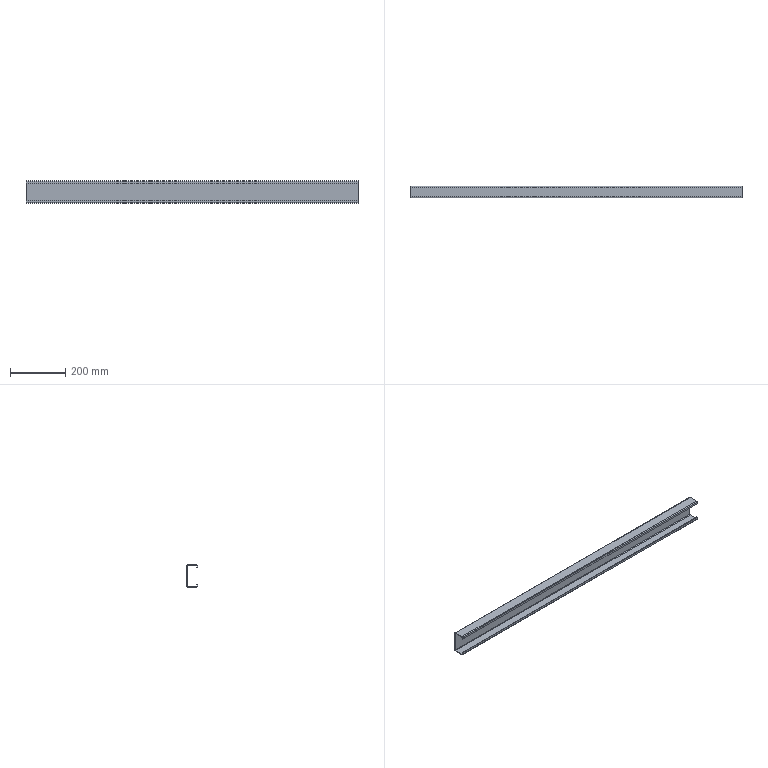Part | SolidWorks | features EdgeFlange 2, FlatPattern 1, SMBaseFlange 1, SheetMetal 1 | 1 solid | 38 faces | box 1200 x 40 x 80 mm | volume 402499 mm3 | plane 30 | cylinder 8 | commonest cylinder face diameters 2 x2 4 x2 6 x2 8 x2
STEP:
#1=CARTESIAN_POINT('',(-1074.379,-37.,-2.));
#2=VERTEX_POINT('',#1);
#3=CARTESIAN_POINT('',(-1074.379,-4.,-2.));
#4=VERTEX_POINT('',#3);
#5=CARTESIAN_POINT('',(-1074.379,0.,-2.));
#6=DIRECTION('',(0.,1.,0.));
#7=VECTOR('',#6,1000.);
#8=LINE('',#5,#7);
#9=EDGE_CURVE('',#2,#4,#8,.T.);
#10=ORIENTED_EDGE('',*,*,#9,.F.);
#11=CARTESIAN_POINT('',(-1074.379,-37.,0.));
#12=VERTEX_POINT('',#11);
#13=CARTESIAN_POINT('',(-1074.379,-37.,-2.));
#14=DIRECTION('',(0.,0.,1.));
#15=VECTOR('',#14,1000.);
#16=LINE('',#13,#15);
#17=EDGE_CURVE('',#2,#12,#16,.T.);
#18=ORIENTED_EDGE('',*,*,#17,.T.);
#19=CARTESIAN_POINT('',(-1074.379,-4.,0.));
#20=VERTEX_POINT('',#19);
#21=CARTESIAN_POINT('',(-1074.379,-2.,0.));
#22=DIRECTION('',(0.,1.,0.));
#23=VECTOR('',#22,1000.);
#24=LINE('',#21,#23);
#25=EDGE_CURVE('',#12,#20,#24,.T.);
#26=ORIENTED_EDGE('',*,*,#25,.T.);
#27=CARTESIAN_POINT('',(-1074.379,-4.,-2.));
#28=DIRECTION('',(0.,0.,1.));
#29=VECTOR('',#28,1000.);
#30=LINE('',#27,#29);
#31=EDGE_CURVE('',#4,#20,#30,.T.);
#32=ORIENTED_EDGE('',*,*,#31,.F.);
#33=EDGE_LOOP('',(#10,#18,#26,#32));
#34=FACE_OUTER_BOUND('',#33,.T.);
#35=CARTESIAN_POINT('',(-1074.379,-2.,0.));
#36=DIRECTION('',(-1.,0.,0.));
#37=DIRECTION('',(0.,0.,1.));
#38=AXIS2_PLACEMENT_3D('',#35,#36,#37);
#39=PLANE('',#38);
#40=ADVANCED_FACE('',(#34),#39,.T.);
#41=ORIENTED_EDGE('',*,*,#25,.F.);
#42=CARTESIAN_POINT('',(125.621,-37.,0.));
#43=VERTEX_POINT('',#42);
#44=CARTESIAN_POINT('',(-1074.379,-37.,0.));
#45=DIRECTION('',(1.,0.,0.));
#46=VECTOR('',#45,1000.);
#47=LINE('',#44,#46);
#48=EDGE_CURVE('',#12,#43,#47,.T.);
#49=ORIENTED_EDGE('',*,*,#48,.T.);
#50=CARTESIAN_POINT('',(125.621,-4.,0.));
#51=VERTEX_POINT('',#50);
#52=CARTESIAN_POINT('',(125.621,-40.,0.));
#53=DIRECTION('',(0.,-1.,0.));
#54=VECTOR('',#53,1000.);
#55=LINE('',#52,#54);
#56=EDGE_CURVE('',#51,#43,#55,.T.);
#57=ORIENTED_EDGE('',*,*,#56,.F.);
#58=CARTESIAN_POINT('',(0.,-4.,0.));
#59=DIRECTION('',(-1.,0.,0.));
#60=VECTOR('',#59,1000.);
#61=LINE('',#58,#60);
#62=EDGE_CURVE('',#51,#20,#61,.T.);
#63=ORIENTED_EDGE('',*,*,#62,.T.);
#64=EDGE_LOOP('',(#41,#49,#57,#63));
#65=FACE_OUTER_BOUND('',#64,.T.);
#66=CARTESIAN_POINT('',(0.,0.,0.));
#67=DIRECTION('',(0.,0.,1.));
#68=DIRECTION('',(0.,-1.,0.));
#69=AXIS2_PLACEMENT_3D('',#66,#67,#68);
#70=PLANE('',#69);
#71=ADVANCED_FACE('',(#65),#70,.T.);
#72=CARTESIAN_POINT('',(125.621,-37.,-2.));
#73=VERTEX_POINT('',#72);
#74=CARTESIAN_POINT('',(-1074.379,-37.,-2.));
#75=DIRECTION('',(1.,0.,0.));
#76=VECTOR('',#75,1000.);
#77=LINE('',#74,#76);
#78=EDGE_CURVE('',#2,#73,#77,.T.);
#79=ORIENTED_EDGE('',*,*,#78,.F.);
#80=ORIENTED_EDGE('',*,*,#9,.T.);
#81=CARTESIAN_POINT('',(125.621,-4.,-2.));
#82=VERTEX_POINT('',#81);
#83=CARTESIAN_POINT('',(125.621,-4.,-2.));
#84=DIRECTION('',(-1.,0.,0.));
#85=VECTOR('',#84,1000.);
#86=LINE('',#83,#85);
#87=EDGE_CURVE('',#82,#4,#86,.T.);
#88=ORIENTED_EDGE('',*,*,#87,.F.);
#89=CARTESIAN_POINT('',(125.621,0.,-2.));
#90=DIRECTION('',(0.,-1.,0.));
#91=VECTOR('',#90,1000.);
#92=LINE('',#89,#91);
#93=EDGE_CURVE('',#82,#73,#92,.T.);
#94=ORIENTED_EDGE('',*,*,#93,.T.);
#95=EDGE_LOOP('',(#79,#80,#88,#94));
#96=FACE_OUTER_BOUND('',#95,.T.);
#97=CARTESIAN_POINT('',(0.,0.,-2.));
#98=DIRECTION('',(0.,0.,1.));
#99=DIRECTION('',(0.,-1.,0.));
#100=AXIS2_PLACEMENT_3D('',#97,#98,#99);
#101=PLANE('',#100);
#102=ADVANCED_FACE('',(#96),#101,.F.);
#103=CARTESIAN_POINT('',(125.621,-37.,-78.));
#104=VERTEX_POINT('',#103);
#105=CARTESIAN_POINT('',(125.621,-4.,-78.));
#106=VERTEX_POINT('',#105);
#107=CARTESIAN_POINT('',(125.621,0.,-78.));
#108=DIRECTION('',(0.,1.,0.));
#109=VECTOR('',#108,1000.);
#110=LINE('',#107,#109);
#111=EDGE_CURVE('',#104,#106,#110,.T.);
#112=ORIENTED_EDGE('',*,*,#111,.F.);
#113=CARTESIAN_POINT('',(125.621,-37.,-80.));
#114=VERTEX_POINT('',#113);
#115=CARTESIAN_POINT('',(125.621,-37.,-78.));
#116=DIRECTION('',(0.,0.,-1.));
#117=VECTOR('',#116,1000.);
#118=LINE('',#115,#117);
#119=EDGE_CURVE('',#104,#114,#118,.T.);
#120=ORIENTED_EDGE('',*,*,#119,.T.);
#121=CARTESIAN_POINT('',(125.621,-4.,-80.));
#122=VERTEX_POINT('',#121);
#123=CARTESIAN_POINT('',(125.621,-2.,-80.));
#124=DIRECTION('',(0.,1.,0.));
#125=VECTOR('',#124,1000.);
#126=LINE('',#123,#125);
#127=EDGE_CURVE('',#114,#122,#126,.T.);
#128=ORIENTED_EDGE('',*,*,#127,.T.);
#129=CARTESIAN_POINT('',(125.621,-4.,-78.));
#130=DIRECTION('',(0.,0.,-1.));
#131=VECTOR('',#130,1000.);
#132=LINE('',#129,#131);
#133=EDGE_CURVE('',#106,#122,#132,.T.);
#134=ORIENTED_EDGE('',*,*,#133,.F.);
#135=EDGE_LOOP('',(#112,#120,#128,#134));
#136=FACE_OUTER_BOUND('',#135,.T.);
#137=CARTESIAN_POINT('',(125.621,-2.,-80.));
#138=DIRECTION('',(1.,0.,0.));
#139=DIRECTION('',(0.,0.,-1.));
#140=AXIS2_PLACEMENT_3D('',#137,#138,#139);
#141=PLANE('',#140);
#142=ADVANCED_FACE('',(#136),#141,.T.);
#143=ORIENTED_EDGE('',*,*,#127,.F.);
#144=CARTESIAN_POINT('',(-1074.379,-37.,-80.));
#145=VERTEX_POINT('',#144);
#146=CARTESIAN_POINT('',(125.621,-37.,-80.));
#147=DIRECTION('',(-1.,0.,0.));
#148=VECTOR('',#147,1000.);
#149=LINE('',#146,#148);
#150=EDGE_CURVE('',#114,#145,#149,.T.);
#151=ORIENTED_EDGE('',*,*,#150,.T.);
#152=CARTESIAN_POINT('',(-1074.379,-4.,-80.));
#153=VERTEX_POINT('',#152);
#154=CARTESIAN_POINT('',(-1074.379,-40.,-80.));
#155=DIRECTION('',(0.,-1.,0.));
#156=VECTOR('',#155,1000.);
#157=LINE('',#154,#156);
#158=EDGE_CURVE('',#153,#145,#157,.T.);
#159=ORIENTED_EDGE('',*,*,#158,.F.);
#160=CARTESIAN_POINT('',(0.,-4.,-80.));
#161=DIRECTION('',(1.,0.,0.));
#162=VECTOR('',#161,1000.);
#163=LINE('',#160,#162);
#164=EDGE_CURVE('',#153,#122,#163,.T.);
#165=ORIENTED_EDGE('',*,*,#164,.T.);
#166=EDGE_LOOP('',(#143,#151,#159,#165));
#167=FACE_OUTER_BOUND('',#166,.T.);
#168=CARTESIAN_POINT('',(0.,0.,-80.));
#169=DIRECTION('',(0.,0.,-1.));
#170=DIRECTION('',(0.,1.,0.));
#171=AXIS2_PLACEMENT_3D('',#168,#169,#170);
#172=PLANE('',#171);
#173=ADVANCED_FACE('',(#167),#172,.T.);
#174=CARTESIAN_POINT('',(-1074.379,-37.,-78.));
#175=VERTEX_POINT('',#174);
#176=CARTESIAN_POINT('',(125.621,-37.,-78.));
#177=DIRECTION('',(-1.,0.,0.));
#178=VECTOR('',#177,1000.);
#179=LINE('',#176,#178);
#180=EDGE_CURVE('',#104,#175,#179,.T.);
#181=ORIENTED_EDGE('',*,*,#180,.F.);
#182=ORIENTED_EDGE('',*,*,#111,.T.);
#183=CARTESIAN_POINT('',(-1074.379,-4.,-78.));
#184=VERTEX_POINT('',#183);
#185=CARTESIAN_POINT('',(-1074.379,-4.,-78.));
#186=DIRECTION('',(1.,0.,0.));
#187=VECTOR('',#186,1000.);
#188=LINE('',#185,#187);
#189=EDGE_CURVE('',#184,#106,#188,.T.);
#190=ORIENTED_EDGE('',*,*,#189,.F.);
#191=CARTESIAN_POINT('',(-1074.379,0.,-78.));
#192=DIRECTION('',(0.,-1.,0.));
#193=VECTOR('',#192,1000.);
#194=LINE('',#191,#193);
#195=EDGE_CURVE('',#184,#175,#194,.T.);
#196=ORIENTED_EDGE('',*,*,#195,.T.);
#197=EDGE_LOOP('',(#181,#182,#190,#196));
#198=FACE_OUTER_BOUND('',#197,.T.);
#199=CARTESIAN_POINT('',(0.,0.,-78.));
#200=DIRECTION('',(0.,0.,-1.));
#201=DIRECTION('',(0.,1.,0.));
#202=AXIS2_PLACEMENT_3D('',#199,#200,#201);
#203=PLANE('',#202);
#204=ADVANCED_FACE('',(#198),#203,.F.);
#205=CARTESIAN_POINT('',(125.621,-2.,-76.));
#206=VERTEX_POINT('',#205);
#207=CARTESIAN_POINT('',(-1074.379,-2.,-76.));
#208=VERTEX_POINT('',#207);
#209=CARTESIAN_POINT('',(125.621,-2.,-76.));
#210=DIRECTION('',(-1.,0.,0.));
#211=VECTOR('',#210,1000.);
#212=LINE('',#209,#211);
#213=EDGE_CURVE('',#206,#208,#212,.T.);
#214=ORIENTED_EDGE('',*,*,#213,.F.);
#215=CARTESIAN_POINT('',(125.621,-2.,-4.));
#216=VERTEX_POINT('',#215);
#217=CARTESIAN_POINT('',(125.621,-2.,-80.));
#218=DIRECTION('',(0.,0.,-1.));
#219=VECTOR('',#218,1000.);
#220=LINE('',#217,#219);
#221=EDGE_CURVE('',#216,#206,#220,.T.);
#222=ORIENTED_EDGE('',*,*,#221,.F.);
#223=CARTESIAN_POINT('',(-1074.379,-2.,-4.));
#224=VERTEX_POINT('',#223);
#225=CARTESIAN_POINT('',(-1074.379,-2.,-4.));
#226=DIRECTION('',(1.,0.,0.));
#227=VECTOR('',#226,1000.);
#228=LINE('',#225,#227);
#229=EDGE_CURVE('',#224,#216,#228,.T.);
#230=ORIENTED_EDGE('',*,*,#229,.F.);
#231=CARTESIAN_POINT('',(-1074.379,-2.,-80.));
#232=DIRECTION('',(0.,0.,1.));
#233=VECTOR('',#232,1000.);
#234=LINE('',#231,#233);
#235=EDGE_CURVE('',#208,#224,#234,.T.);
#236=ORIENTED_EDGE('',*,*,#235,.F.);
#237=EDGE_LOOP('',(#214,#222,#230,#236));
#238=FACE_OUTER_BOUND('',#237,.T.);
#239=CARTESIAN_POINT('',(0.,-2.,0.));
#240=DIRECTION('',(0.,1.,0.));
#241=DIRECTION('',(0.,0.,1.));
#242=AXIS2_PLACEMENT_3D('',#239,#240,#241);
#243=PLANE('',#242);
#244=ADVANCED_FACE('',(#238),#243,.F.);
#245=CARTESIAN_POINT('',(125.621,0.,-4.));
#246=VERTEX_POINT('',#245);
#247=CARTESIAN_POINT('',(125.621,0.,-76.));
#248=VERTEX_POINT('',#247);
#249=CARTESIAN_POINT('',(125.621,0.,-80.));
#250=DIRECTION('',(0.,0.,-1.));
#251=VECTOR('',#250,1000.);
#252=LINE('',#249,#251);
#253=EDGE_CURVE('',#246,#248,#252,.T.);
#254=ORIENTED_EDGE('',*,*,#253,.T.);
#255=CARTESIAN_POINT('',(-1074.379,0.,-76.));
#256=VERTEX_POINT('',#255);
#257=CARTESIAN_POINT('',(125.621,0.,-76.));
#258=DIRECTION('',(-1.,0.,0.));
#259=VECTOR('',#258,1000.);
#260=LINE('',#257,#259);
#261=EDGE_CURVE('',#248,#256,#260,.T.);
#262=ORIENTED_EDGE('',*,*,#261,.T.);
#263=CARTESIAN_POINT('',(-1074.379,0.,-4.));
#264=VERTEX_POINT('',#263);
#265=CARTESIAN_POINT('',(-1074.379,0.,-80.));
#266=DIRECTION('',(0.,0.,1.));
#267=VECTOR('',#266,1000.);
#268=LINE('',#265,#267);
#269=EDGE_CURVE('',#256,#264,#268,.T.);
#270=ORIENTED_EDGE('',*,*,#269,.T.);
#271=CARTESIAN_POINT('',(-1074.379,0.,-4.));
#272=DIRECTION('',(1.,0.,0.));
#273=VECTOR('',#272,1000.);
#274=LINE('',#271,#273);
#275=EDGE_CURVE('',#264,#246,#274,.T.);
#276=ORIENTED_EDGE('',*,*,#275,.T.);
#277=EDGE_LOOP('',(#254,#262,#270,#276));
#278=FACE_OUTER_BOUND('',#277,.T.);
#279=CARTESIAN_POINT('',(0.,0.,0.));
#280=DIRECTION('',(0.,1.,0.));
#281=DIRECTION('',(0.,0.,1.));
#282=AXIS2_PLACEMENT_3D('',#279,#280,#281);
#283=PLANE('',#282);
#284=ADVANCED_FACE('',(#278),#283,.T.);
#285=ORIENTED_EDGE('',*,*,#221,.T.);
#286=CARTESIAN_POINT('',(125.621,-2.,-76.));
#287=DIRECTION('',(0.,1.,0.));
#288=VECTOR('',#287,1000.);
#289=LINE('',#286,#288);
#290=EDGE_CURVE('',#206,#248,#289,.T.);
#291=ORIENTED_EDGE('',*,*,#290,.T.);
#292=ORIENTED_EDGE('',*,*,#253,.F.);
#293=CARTESIAN_POINT('',(125.621,-2.,-4.));
#294=DIRECTION('',(0.,1.,0.));
#295=VECTOR('',#294,1000.);
#296=LINE('',#293,#295);
#297=EDGE_CURVE('',#216,#246,#296,.T.);
#298=ORIENTED_EDGE('',*,*,#297,.F.);
#299=EDGE_LOOP('',(#285,#291,#292,#298));
#300=FACE_OUTER_BOUND('',#299,.T.);
#301=CARTESIAN_POINT('',(125.621,-2.,-80.));
#302=DIRECTION('',(1.,0.,0.));
#303=DIRECTION('',(0.,0.,-1.));
#304=AXIS2_PLACEMENT_3D('',#301,#302,#303);
#305=PLANE('',#304);
#306=ADVANCED_FACE('',(#300),#305,.T.);
#307=CARTESIAN_POINT('',(-1074.379,-2.,-76.));
#308=DIRECTION('',(0.,1.,0.));
#309=VECTOR('',#308,1000.);
#310=LINE('',#307,#309);
#311=EDGE_CURVE('',#208,#256,#310,.T.);
#312=ORIENTED_EDGE('',*,*,#311,.F.);
#313=ORIENTED_EDGE('',*,*,#235,.T.);
#314=CARTESIAN_POINT('',(-1074.379,-2.,-4.));
#315=DIRECTION('',(0.,1.,0.));
#316=VECTOR('',#315,1000.);
#317=LINE('',#314,#316);
#318=EDGE_CURVE('',#224,#264,#317,.T.);
#319=ORIENTED_EDGE('',*,*,#318,.T.);
#320=ORIENTED_EDGE('',*,*,#269,.F.);
#321=EDGE_LOOP('',(#312,#313,#319,#320));
#322=FACE_OUTER_BOUND('',#321,.T.);
#323=CARTESIAN_POINT('',(-1074.379,-2.,-80.));
#324=DIRECTION('',(-1.,0.,0.));
#325=DIRECTION('',(0.,0.,1.));
#326=AXIS2_PLACEMENT_3D('',#323,#324,#325);
#327=PLANE('',#326);
#328=ADVANCED_FACE('',(#322),#327,.T.);
#329=CARTESIAN_POINT('',(125.621,-4.,0.));
#330=DIRECTION('',(0.,0.,1.));
#331=VECTOR('',#330,1000.);
#332=LINE('',#329,#331);
#333=EDGE_CURVE('',#82,#51,#332,.T.);
#334=ORIENTED_EDGE('',*,*,#333,.F.);
#335=CARTESIAN_POINT('',(125.621,-4.,-4.));
#336=DIRECTION('',(1.,0.,0.));
#337=DIRECTION('',(0.,0.,1.));
#338=AXIS2_PLACEMENT_3D('',#335,#336,#337);
#339=CIRCLE('',#338,2.);
#340=EDGE_CURVE('',#216,#82,#339,.T.);
#341=ORIENTED_EDGE('',*,*,#340,.F.);
#342=ORIENTED_EDGE('',*,*,#297,.T.);
#343=CARTESIAN_POINT('',(125.621,-4.,-4.));
#344=DIRECTION('',(1.,0.,0.));
#345=DIRECTION('',(0.,0.,1.));
#346=AXIS2_PLACEMENT_3D('',#343,#344,#345);
#347=CIRCLE('',#346,4.);
#348=EDGE_CURVE('',#246,#51,#347,.T.);
#349=ORIENTED_EDGE('',*,*,#348,.T.);
#350=EDGE_LOOP('',(#334,#341,#342,#349));
#351=FACE_OUTER_BOUND('',#350,.T.);
#352=CARTESIAN_POINT('',(125.621,-4.,-4.));
#353=DIRECTION('',(1.,0.,0.));
#354=DIRECTION('',(0.,0.,-1.));
#355=AXIS2_PLACEMENT_3D('',#352,#353,#354);
#356=PLANE('',#355);
#357=ADVANCED_FACE('',(#351),#356,.T.);
#358=CARTESIAN_POINT('',(-1074.379,-4.,-4.));
#359=DIRECTION('',(-1.,0.,0.));
#360=DIRECTION('',(0.,0.,1.));
#361=AXIS2_PLACEMENT_3D('',#358,#359,#360);
#362=CIRCLE('',#361,2.);
#363=EDGE_CURVE('',#4,#224,#362,.T.);
#364=ORIENTED_EDGE('',*,*,#363,.F.);
#365=ORIENTED_EDGE('',*,*,#31,.T.);
#366=CARTESIAN_POINT('',(-1074.379,-4.,-4.));
#367=DIRECTION('',(-1.,0.,0.));
#368=DIRECTION('',(0.,0.,1.));
#369=AXIS2_PLACEMENT_3D('',#366,#367,#368);
#370=CIRCLE('',#369,4.);
#371=EDGE_CURVE('',#20,#264,#370,.T.);
#372=ORIENTED_EDGE('',*,*,#371,.T.);
#373=ORIENTED_EDGE('',*,*,#318,.F.);
#374=EDGE_LOOP('',(#364,#365,#372,#373));
#375=FACE_OUTER_BOUND('',#374,.T.);
#376=CARTESIAN_POINT('',(-1074.379,-4.,-4.));
#377=DIRECTION('',(1.,0.,0.));
#378=DIRECTION('',(0.,0.,-1.));
#379=AXIS2_PLACEMENT_3D('',#376,#377,#378);
#380=PLANE('',#379);
#381=ADVANCED_FACE('',(#375),#380,.F.);
#382=ORIENTED_EDGE('',*,*,#275,.F.);
#383=ORIENTED_EDGE('',*,*,#371,.F.);
#384=ORIENTED_EDGE('',*,*,#62,.F.);
#385=ORIENTED_EDGE('',*,*,#348,.F.);
#386=EDGE_LOOP('',(#382,#383,#384,#385));
#387=FACE_OUTER_BOUND('',#386,.T.);
#388=CARTESIAN_POINT('',(-1074.379,-4.,-4.));
#389=DIRECTION('',(-1.,0.,0.));
#390=DIRECTION('',(0.,0.,1.));
#391=AXIS2_PLACEMENT_3D('',#388,#389,#390);
#392=CYLINDRICAL_SURFACE('',#391,4.);
#393=ADVANCED_FACE('',(#387),#392,.T.);
#394=ORIENTED_EDGE('',*,*,#229,.T.);
#395=ORIENTED_EDGE('',*,*,#340,.T.);
#396=ORIENTED_EDGE('',*,*,#87,.T.);
#397=ORIENTED_EDGE('',*,*,#363,.T.);
#398=EDGE_LOOP('',(#394,#395,#396,#397));
#399=FACE_OUTER_BOUND('',#398,.T.);
#400=CARTESIAN_POINT('',(-1074.379,-4.,-4.));
#401=DIRECTION('',(-1.,0.,0.));
#402=DIRECTION('',(0.,0.,1.));
#403=AXIS2_PLACEMENT_3D('',#400,#401,#402);
#404=CYLINDRICAL_SURFACE('',#403,2.);
#405=ADVANCED_FACE('',(#399),#404,.F.);
#406=CARTESIAN_POINT('',(125.621,-37.,-2.));
#407=DIRECTION('',(0.,0.,1.));
#408=VECTOR('',#407,1000.);
#409=LINE('',#406,#408);
#410=EDGE_CURVE('',#73,#43,#409,.T.);
#411=ORIENTED_EDGE('',*,*,#410,.F.);
#412=ORIENTED_EDGE('',*,*,#93,.F.);
#413=ORIENTED_EDGE('',*,*,#333,.T.);
#414=ORIENTED_EDGE('',*,*,#56,.T.);
#415=EDGE_LOOP('',(#411,#412,#413,#414));
#416=FACE_OUTER_BOUND('',#415,.T.);
#417=CARTESIAN_POINT('',(125.621,-40.,0.));
#418=DIRECTION('',(1.,0.,0.));
#419=DIRECTION('',(0.,0.,-1.));
#420=AXIS2_PLACEMENT_3D('',#417,#418,#419);
#421=PLANE('',#420);
#422=ADVANCED_FACE('',(#416),#421,.T.);
#423=CARTESIAN_POINT('',(-1074.379,-4.,-80.));
#424=DIRECTION('',(0.,0.,-1.));
#425=VECTOR('',#424,1000.);
#426=LINE('',#423,#425);
#427=EDGE_CURVE('',#184,#153,#426,.T.);
#428=ORIENTED_EDGE('',*,*,#427,.F.);
#429=CARTESIAN_POINT('',(-1074.379,-4.,-76.));
#430=DIRECTION('',(-1.,0.,0.));
#431=DIRECTION('',(0.,0.,-1.));
#432=AXIS2_PLACEMENT_3D('',#429,#430,#431);
#433=CIRCLE('',#432,2.);
#434=EDGE_CURVE('',#208,#184,#433,.T.);
#435=ORIENTED_EDGE('',*,*,#434,.F.);
#436=ORIENTED_EDGE('',*,*,#311,.T.);
#437=CARTESIAN_POINT('',(-1074.379,-4.,-76.));
#438=DIRECTION('',(-1.,0.,0.));
#439=DIRECTION('',(0.,0.,-1.));
#440=AXIS2_PLACEMENT_3D('',#437,#438,#439);
#441=CIRCLE('',#440,4.);
#442=EDGE_CURVE('',#256,#153,#441,.T.);
#443=ORIENTED_EDGE('',*,*,#442,.T.);
#444=EDGE_LOOP('',(#428,#435,#436,#443));
#445=FACE_OUTER_BOUND('',#444,.T.);
#446=CARTESIAN_POINT('',(-1074.379,-4.,-76.));
#447=DIRECTION('',(-1.,0.,0.));
#448=DIRECTION('',(0.,0.,1.));
#449=AXIS2_PLACEMENT_3D('',#446,#447,#448);
#450=PLANE('',#449);
#451=ADVANCED_FACE('',(#445),#450,.T.);
#452=CARTESIAN_POINT('',(125.621,-4.,-76.));
#453=DIRECTION('',(1.,0.,0.));
#454=DIRECTION('',(0.,0.,-1.));
#455=AXIS2_PLACEMENT_3D('',#452,#453,#454);
#456=CIRCLE('',#455,2.);
#457=EDGE_CURVE('',#106,#206,#456,.T.);
#458=ORIENTED_EDGE('',*,*,#457,.F.);
#459=ORIENTED_EDGE('',*,*,#133,.T.);
#460=CARTESIAN_POINT('',(125.621,-4.,-76.));
#461=DIRECTION('',(1.,0.,0.));
#462=DIRECTION('',(0.,0.,-1.));
#463=AXIS2_PLACEMENT_3D('',#460,#461,#462);
#464=CIRCLE('',#463,4.);
#465=EDGE_CURVE('',#122,#248,#464,.T.);
#466=ORIENTED_EDGE('',*,*,#465,.T.);
#467=ORIENTED_EDGE('',*,*,#290,.F.);
#468=EDGE_LOOP('',(#458,#459,#466,#467));
#469=FACE_OUTER_BOUND('',#468,.T.);
#470=CARTESIAN_POINT('',(125.621,-4.,-76.));
#471=DIRECTION('',(-1.,0.,0.));
#472=DIRECTION('',(0.,0.,1.));
#473=AXIS2_PLACEMENT_3D('',#470,#471,#472);
#474=PLANE('',#473);
#475=ADVANCED_FACE('',(#469),#474,.F.);
#476=ORIENTED_EDGE('',*,*,#261,.F.);
#477=ORIENTED_EDGE('',*,*,#465,.F.);
#478=ORIENTED_EDGE('',*,*,#164,.F.);
#479=ORIENTED_EDGE('',*,*,#442,.F.);
#480=EDGE_LOOP('',(#476,#477,#478,#479));
#481=FACE_OUTER_BOUND('',#480,.T.);
#482=CARTESIAN_POINT('',(125.621,-4.,-76.));
#483=DIRECTION('',(1.,0.,0.));
#484=DIRECTION('',(0.,0.,-1.));
#485=AXIS2_PLACEMENT_3D('',#482,#483,#484);
#486=CYLINDRICAL_SURFACE('',#485,4.);
#487=ADVANCED_FACE('',(#481),#486,.T.);
#488=ORIENTED_EDGE('',*,*,#213,.T.);
#489=ORIENTED_EDGE('',*,*,#434,.T.);
#490=ORIENTED_EDGE('',*,*,#189,.T.);
#491=ORIENTED_EDGE('',*,*,#457,.T.);
#492=EDGE_LOOP('',(#488,#489,#490,#491));
#493=FACE_OUTER_BOUND('',#492,.T.);
#494=CARTESIAN_POINT('',(125.621,-4.,-76.));
#495=DIRECTION('',(1.,0.,0.));
#496=DIRECTION('',(0.,0.,-1.));
#497=AXIS2_PLACEMENT_3D('',#494,#495,#496);
#498=CYLINDRICAL_SURFACE('',#497,2.);
#499=ADVANCED_FACE('',(#493),#498,.F.);
#500=CARTESIAN_POINT('',(-1074.379,-37.,-78.));
#501=DIRECTION('',(0.,0.,-1.));
#502=VECTOR('',#501,1000.);
#503=LINE('',#500,#502);
#504=EDGE_CURVE('',#175,#145,#503,.T.);
#505=ORIENTED_EDGE('',*,*,#504,.F.);
#506=ORIENTED_EDGE('',*,*,#195,.F.);
#507=ORIENTED_EDGE('',*,*,#427,.T.);
#508=ORIENTED_EDGE('',*,*,#158,.T.);
#509=EDGE_LOOP('',(#505,#506,#507,#508));
#510=FACE_OUTER_BOUND('',#509,.T.);
#511=CARTESIAN_POINT('',(-1074.379,-40.,-80.));
#512=DIRECTION('',(-1.,0.,0.));
#513=DIRECTION('',(0.,0.,1.));
#514=AXIS2_PLACEMENT_3D('',#511,#512,#513);
#515=PLANE('',#514);
#516=ADVANCED_FACE('',(#510),#515,.T.);
#517=CARTESIAN_POINT('',(-1074.379,-38.,-77.));
#518=VERTEX_POINT('',#517);
#519=CARTESIAN_POINT('',(-1074.379,-40.,-77.));
#520=VERTEX_POINT('',#519);
#521=CARTESIAN_POINT('',(-1074.379,-40.,-77.));
#522=DIRECTION('',(0.,-1.,0.));
#523=VECTOR('',#522,1000.);
#524=LINE('',#521,#523);
#525=EDGE_CURVE('',#518,#520,#524,.T.);
#526=ORIENTED_EDGE('',*,*,#525,.F.);
#527=CARTESIAN_POINT('',(-1074.379,-37.,-77.));
#528=DIRECTION('',(-1.,0.,0.));
#529=DIRECTION('',(0.,0.,-1.));
#530=AXIS2_PLACEMENT_3D('',#527,#528,#529);
#531=CIRCLE('',#530,1.);
#532=EDGE_CURVE('',#175,#518,#531,.T.);
#533=ORIENTED_EDGE('',*,*,#532,.F.);
#534=ORIENTED_EDGE('',*,*,#504,.T.);
#535=CARTESIAN_POINT('',(-1074.379,-37.,-77.));
#536=DIRECTION('',(-1.,0.,0.));
#537=DIRECTION('',(0.,0.,-1.));
#538=AXIS2_PLACEMENT_3D('',#535,#536,#537);
#539=CIRCLE('',#538,3.);
#540=EDGE_CURVE('',#145,#520,#539,.T.);
#541=ORIENTED_EDGE('',*,*,#540,.T.);
#542=EDGE_LOOP('',(#526,#533,#534,#541));
#543=FACE_OUTER_BOUND('',#542,.T.);
#544=CARTESIAN_POINT('',(-1074.379,-37.,-77.));
#545=DIRECTION('',(-1.,0.,0.));
#546=DIRECTION('',(0.,0.,1.));
#547=AXIS2_PLACEMENT_3D('',#544,#545,#546);
#548=PLANE('',#547);
#549=ADVANCED_FACE('',(#543),#548,.T.);
#550=CARTESIAN_POINT('',(125.621,-38.,-77.));
#551=VERTEX_POINT('',#550);
#552=CARTESIAN_POINT('',(125.621,-37.,-77.));
#553=DIRECTION('',(1.,0.,0.));
#554=DIRECTION('',(0.,0.,-1.));
#555=AXIS2_PLACEMENT_3D('',#552,#553,#554);
#556=CIRCLE('',#555,1.);
#557=EDGE_CURVE('',#551,#104,#556,.T.);
#558=ORIENTED_EDGE('',*,*,#557,.F.);
#559=CARTESIAN_POINT('',(125.621,-40.,-77.));
#560=VERTEX_POINT('',#559);
#561=CARTESIAN_POINT('',(125.621,-38.,-77.));
#562=DIRECTION('',(0.,-1.,0.));
#563=VECTOR('',#562,1000.);
#564=LINE('',#561,#563);
#565=EDGE_CURVE('',#551,#560,#564,.T.);
#566=ORIENTED_EDGE('',*,*,#565,.T.);
#567=CARTESIAN_POINT('',(125.621,-37.,-77.));
#568=DIRECTION('',(1.,0.,0.));
#569=DIRECTION('',(0.,0.,-1.));
#570=AXIS2_PLACEMENT_3D('',#567,#568,#569);
#571=CIRCLE('',#570,3.);
#572=EDGE_CURVE('',#560,#114,#571,.T.);
#573=ORIENTED_EDGE('',*,*,#572,.T.);
#574=ORIENTED_EDGE('',*,*,#119,.F.);
#575=EDGE_LOOP('',(#558,#566,#573,#574));
#576=FACE_OUTER_BOUND('',#575,.T.);
#577=CARTESIAN_POINT('',(125.621,-37.,-77.));
#578=DIRECTION('',(-1.,0.,0.));
#579=DIRECTION('',(0.,0.,1.));
#580=AXIS2_PLACEMENT_3D('',#577,#578,#579);
#581=PLANE('',#580);
#582=ADVANCED_FACE('',(#576),#581,.F.);
#583=ORIENTED_EDGE('',*,*,#150,.F.);
#584=ORIENTED_EDGE('',*,*,#572,.F.);
#585=CARTESIAN_POINT('',(-1074.379,-40.,-77.));
#586=DIRECTION('',(-1.,0.,0.));
#587=VECTOR('',#586,1000.);
#588=LINE('',#585,#587);
#589=EDGE_CURVE('',#560,#520,#588,.T.);
#590=ORIENTED_EDGE('',*,*,#589,.T.);
#591=ORIENTED_EDGE('',*,*,#540,.F.);
#592=EDGE_LOOP('',(#583,#584,#590,#591));
#593=FACE_OUTER_BOUND('',#592,.T.);
#594=CARTESIAN_POINT('',(125.621,-37.,-77.));
#595=DIRECTION('',(1.,0.,0.));
#596=DIRECTION('',(0.,-1.,0.));
#597=AXIS2_PLACEMENT_3D('',#594,#595,#596);
#598=CYLINDRICAL_SURFACE('',#597,3.);
#599=ADVANCED_FACE('',(#593),#598,.T.);
#600=ORIENTED_EDGE('',*,*,#180,.T.);
#601=ORIENTED_EDGE('',*,*,#532,.T.);
#602=CARTESIAN_POINT('',(-1074.379,-38.,-77.));
#603=DIRECTION('',(1.,0.,0.));
#604=VECTOR('',#603,1000.);
#605=LINE('',#602,#604);
#606=EDGE_CURVE('',#518,#551,#605,.T.);
#607=ORIENTED_EDGE('',*,*,#606,.T.);
#608=ORIENTED_EDGE('',*,*,#557,.T.);
#609=EDGE_LOOP('',(#600,#601,#607,#608));
#610=FACE_OUTER_BOUND('',#609,.T.);
#611=CARTESIAN_POINT('',(125.621,-37.,-77.));
#612=DIRECTION('',(1.,0.,0.));
#613=DIRECTION('',(0.,-1.,0.));
#614=AXIS2_PLACEMENT_3D('',#611,#612,#613);
#615=CYLINDRICAL_SURFACE('',#614,1.);
#616=ADVANCED_FACE('',(#610),#615,.F.);
#617=ORIENTED_EDGE('',*,*,#565,.F.);
#618=CARTESIAN_POINT('',(125.621,-38.,-70.));
#619=VERTEX_POINT('',#618);
#620=CARTESIAN_POINT('',(125.621,-38.,-70.));
#621=DIRECTION('',(0.,0.,1.));
#622=VECTOR('',#621,1000.);
#623=LINE('',#620,#622);
#624=EDGE_CURVE('',#551,#619,#623,.T.);
#625=ORIENTED_EDGE('',*,*,#624,.T.);
#626=CARTESIAN_POINT('',(125.621,-40.,-70.));
#627=VERTEX_POINT('',#626);
#628=CARTESIAN_POINT('',(125.621,-40.,-70.));
#629=DIRECTION('',(0.,1.,0.));
#630=VECTOR('',#629,1000.);
#631=LINE('',#628,#630);
#632=EDGE_CURVE('',#627,#619,#631,.T.);
#633=ORIENTED_EDGE('',*,*,#632,.F.);
#634=CARTESIAN_POINT('',(125.621,-40.,0.));
#635=DIRECTION('',(0.,0.,1.));
#636=VECTOR('',#635,1000.);
#637=LINE('',#634,#636);
#638=EDGE_CURVE('',#560,#627,#637,.T.);
#639=ORIENTED_EDGE('',*,*,#638,.F.);
#640=EDGE_LOOP('',(#617,#625,#633,#639));
#641=FACE_OUTER_BOUND('',#640,.T.);
#642=CARTESIAN_POINT('',(125.621,-40.,-70.));
#643=DIRECTION('',(-1.,0.,0.));
#644=DIRECTION('',(0.,-1.,0.));
#645=AXIS2_PLACEMENT_3D('',#642,#643,#644);
#646=PLANE('',#645);
#647=ADVANCED_FACE('',(#641),#646,.F.);
#648=ORIENTED_EDGE('',*,*,#525,.T.);
#649=CARTESIAN_POINT('',(-1074.379,-40.,-70.));
#650=VERTEX_POINT('',#649);
#651=CARTESIAN_POINT('',(-1074.379,-40.,0.));
#652=DIRECTION('',(0.,0.,-1.));
#653=VECTOR('',#652,1000.);
#654=LINE('',#651,#653);
#655=EDGE_CURVE('',#650,#520,#654,.T.);
#656=ORIENTED_EDGE('',*,*,#655,.F.);
#657=CARTESIAN_POINT('',(-1074.379,-38.,-70.));
#658=VERTEX_POINT('',#657);
#659=CARTESIAN_POINT('',(-1074.379,-40.,-70.));
#660=DIRECTION('',(0.,1.,0.));
#661=VECTOR('',#660,1000.);
#662=LINE('',#659,#661);
#663=EDGE_CURVE('',#650,#658,#662,.T.);
#664=ORIENTED_EDGE('',*,*,#663,.T.);
#665=CARTESIAN_POINT('',(-1074.379,-38.,-78.));
#666=DIRECTION('',(0.,0.,-1.));
#667=VECTOR('',#666,1000.);
#668=LINE('',#665,#667);
#669=EDGE_CURVE('',#658,#518,#668,.T.);
#670=ORIENTED_EDGE('',*,*,#669,.T.);
#671=EDGE_LOOP('',(#648,#656,#664,#670));
#672=FACE_OUTER_BOUND('',#671,.T.);
#673=CARTESIAN_POINT('',(-1074.379,-40.,-78.));
#674=DIRECTION('',(1.,0.,0.));
#675=DIRECTION('',(0.,1.,0.));
#676=AXIS2_PLACEMENT_3D('',#673,#674,#675);
#677=PLANE('',#676);
#678=ADVANCED_FACE('',(#672),#677,.F.);
#679=ORIENTED_EDGE('',*,*,#589,.F.);
#680=ORIENTED_EDGE('',*,*,#638,.T.);
#681=CARTESIAN_POINT('',(0.,-40.,-70.));
#682=DIRECTION('',(-1.,0.,0.));
#683=VECTOR('',#682,1000.);
#684=LINE('',#681,#683);
#685=EDGE_CURVE('',#627,#650,#684,.T.);
#686=ORIENTED_EDGE('',*,*,#685,.T.);
#687=ORIENTED_EDGE('',*,*,#655,.T.);
#688=EDGE_LOOP('',(#679,#680,#686,#687));
#689=FACE_OUTER_BOUND('',#688,.T.);
#690=CARTESIAN_POINT('',(0.,-40.,0.));
#691=DIRECTION('',(0.,1.,0.));
#692=DIRECTION('',(0.,0.,1.));
#693=AXIS2_PLACEMENT_3D('',#690,#691,#692);
#694=PLANE('',#693);
#695=ADVANCED_FACE('',(#689),#694,.F.);
#696=ORIENTED_EDGE('',*,*,#624,.F.);
#697=ORIENTED_EDGE('',*,*,#606,.F.);
#698=ORIENTED_EDGE('',*,*,#669,.F.);
#699=CARTESIAN_POINT('',(-1074.379,-38.,-70.));
#700=DIRECTION('',(-1.,0.,0.));
#701=VECTOR('',#700,1000.);
#702=LINE('',#699,#701);
#703=EDGE_CURVE('',#619,#658,#702,.T.);
#704=ORIENTED_EDGE('',*,*,#703,.F.);
#705=EDGE_LOOP('',(#696,#697,#698,#704));
#706=FACE_OUTER_BOUND('',#705,.T.);
#707=CARTESIAN_POINT('',(0.,-38.,0.));
#708=DIRECTION('',(0.,1.,0.));
#709=DIRECTION('',(0.,0.,1.));
#710=AXIS2_PLACEMENT_3D('',#707,#708,#709);
#711=PLANE('',#710);
#712=ADVANCED_FACE('',(#706),#711,.T.);
#713=ORIENTED_EDGE('',*,*,#703,.T.);
#714=ORIENTED_EDGE('',*,*,#663,.F.);
#715=ORIENTED_EDGE('',*,*,#685,.F.);
#716=ORIENTED_EDGE('',*,*,#632,.T.);
#717=EDGE_LOOP('',(#713,#714,#715,#716));
#718=FACE_OUTER_BOUND('',#717,.T.);
#719=CARTESIAN_POINT('',(-1074.379,-40.,-70.));
#720=DIRECTION('',(0.,0.,-1.));
#721=DIRECTION('',(0.,1.,0.));
#722=AXIS2_PLACEMENT_3D('',#719,#720,#721);
#723=PLANE('',#722);
#724=ADVANCED_FACE('',(#718),#723,.F.);
#725=CARTESIAN_POINT('',(125.621,-38.,-3.));
#726=VERTEX_POINT('',#725);
#727=CARTESIAN_POINT('',(125.621,-40.,-3.));
#728=VERTEX_POINT('',#727);
#729=CARTESIAN_POINT('',(125.621,-40.,-3.));
#730=DIRECTION('',(0.,-1.,0.));
#731=VECTOR('',#730,1000.);
#732=LINE('',#729,#731);
#733=EDGE_CURVE('',#726,#728,#732,.T.);
#734=ORIENTED_EDGE('',*,*,#733,.F.);
#735=CARTESIAN_POINT('',(125.621,-37.,-3.));
#736=DIRECTION('',(1.,0.,0.));
#737=DIRECTION('',(0.,0.,1.));
#738=AXIS2_PLACEMENT_3D('',#735,#736,#737);
#739=CIRCLE('',#738,1.);
#740=EDGE_CURVE('',#73,#726,#739,.T.);
#741=ORIENTED_EDGE('',*,*,#740,.F.);
#742=ORIENTED_EDGE('',*,*,#410,.T.);
#743=CARTESIAN_POINT('',(125.621,-37.,-3.));
#744=DIRECTION('',(1.,0.,0.));
#745=DIRECTION('',(0.,0.,1.));
#746=AXIS2_PLACEMENT_3D('',#743,#744,#745);
#747=CIRCLE('',#746,3.);
#748=EDGE_CURVE('',#43,#728,#747,.T.);
#749=ORIENTED_EDGE('',*,*,#748,.T.);
#750=EDGE_LOOP('',(#734,#741,#742,#749));
#751=FACE_OUTER_BOUND('',#750,.T.);
#752=CARTESIAN_POINT('',(125.621,-37.,-3.));
#753=DIRECTION('',(1.,0.,0.));
#754=DIRECTION('',(0.,0.,-1.));
#755=AXIS2_PLACEMENT_3D('',#752,#753,#754);
#756=PLANE('',#755);
#757=ADVANCED_FACE('',(#751),#756,.T.);
#758=CARTESIAN_POINT('',(-1074.379,-38.,-3.));
#759=VERTEX_POINT('',#758);
#760=CARTESIAN_POINT('',(-1074.379,-37.,-3.));
#761=DIRECTION('',(-1.,0.,0.));
#762=DIRECTION('',(0.,0.,1.));
#763=AXIS2_PLACEMENT_3D('',#760,#761,#762);
#764=CIRCLE('',#763,1.);
#765=EDGE_CURVE('',#759,#2,#764,.T.);
#766=ORIENTED_EDGE('',*,*,#765,.F.);
#767=CARTESIAN_POINT('',(-1074.379,-40.,-3.));
#768=VERTEX_POINT('',#767);
#769=CARTESIAN_POINT('',(-1074.379,-38.,-3.));
#770=DIRECTION('',(0.,-1.,0.));
#771=VECTOR('',#770,1000.);
#772=LINE('',#769,#771);
#773=EDGE_CURVE('',#759,#768,#772,.T.);
#774=ORIENTED_EDGE('',*,*,#773,.T.);
#775=CARTESIAN_POINT('',(-1074.379,-37.,-3.));
#776=DIRECTION('',(-1.,0.,0.));
#777=DIRECTION('',(0.,0.,1.));
#778=AXIS2_PLACEMENT_3D('',#775,#776,#777);
#779=CIRCLE('',#778,3.);
#780=EDGE_CURVE('',#768,#12,#779,.T.);
#781=ORIENTED_EDGE('',*,*,#780,.T.);
#782=ORIENTED_EDGE('',*,*,#17,.F.);
#783=EDGE_LOOP('',(#766,#774,#781,#782));
#784=FACE_OUTER_BOUND('',#783,.T.);
#785=CARTESIAN_POINT('',(-1074.379,-37.,-3.));
#786=DIRECTION('',(1.,0.,0.));
#787=DIRECTION('',(0.,0.,-1.));
#788=AXIS2_PLACEMENT_3D('',#785,#786,#787);
#789=PLANE('',#788);
#790=ADVANCED_FACE('',(#784),#789,.F.);
#791=ORIENTED_EDGE('',*,*,#48,.F.);
#792=ORIENTED_EDGE('',*,*,#780,.F.);
#793=CARTESIAN_POINT('',(125.621,-40.,-3.));
#794=DIRECTION('',(1.,0.,0.));
#795=VECTOR('',#794,1000.);
#796=LINE('',#793,#795);
#797=EDGE_CURVE('',#768,#728,#796,.T.);
#798=ORIENTED_EDGE('',*,*,#797,.T.);
#799=ORIENTED_EDGE('',*,*,#748,.F.);
#800=EDGE_LOOP('',(#791,#792,#798,#799));
#801=FACE_OUTER_BOUND('',#800,.T.);
#802=CARTESIAN_POINT('',(-1074.379,-37.,-3.));
#803=DIRECTION('',(-1.,0.,0.));
#804=DIRECTION('',(0.,-1.,0.));
#805=AXIS2_PLACEMENT_3D('',#802,#803,#804);
#806=CYLINDRICAL_SURFACE('',#805,3.);
#807=ADVANCED_FACE('',(#801),#806,.T.);
#808=ORIENTED_EDGE('',*,*,#78,.T.);
#809=ORIENTED_EDGE('',*,*,#740,.T.);
#810=CARTESIAN_POINT('',(125.621,-38.,-3.));
#811=DIRECTION('',(-1.,0.,0.));
#812=VECTOR('',#811,1000.);
#813=LINE('',#810,#812);
#814=EDGE_CURVE('',#726,#759,#813,.T.);
#815=ORIENTED_EDGE('',*,*,#814,.T.);
#816=ORIENTED_EDGE('',*,*,#765,.T.);
#817=EDGE_LOOP('',(#808,#809,#815,#816));
#818=FACE_OUTER_BOUND('',#817,.T.);
#819=CARTESIAN_POINT('',(-1074.379,-37.,-3.));
#820=DIRECTION('',(-1.,0.,0.));
#821=DIRECTION('',(0.,-1.,0.));
#822=AXIS2_PLACEMENT_3D('',#819,#820,#821);
#823=CYLINDRICAL_SURFACE('',#822,1.);
#824=ADVANCED_FACE('',(#818),#823,.F.);
#825=ORIENTED_EDGE('',*,*,#733,.T.);
#826=CARTESIAN_POINT('',(125.621,-40.,-10.));
#827=VERTEX_POINT('',#826);
#828=CARTESIAN_POINT('',(125.621,-40.,0.));
#829=DIRECTION('',(0.,0.,1.));
#830=VECTOR('',#829,1000.);
#831=LINE('',#828,#830);
#832=EDGE_CURVE('',#827,#728,#831,.T.);
#833=ORIENTED_EDGE('',*,*,#832,.F.);
#834=CARTESIAN_POINT('',(125.621,-38.,-10.));
#835=VERTEX_POINT('',#834);
#836=CARTESIAN_POINT('',(125.621,-40.,-10.));
#837=DIRECTION('',(0.,1.,0.));
#838=VECTOR('',#837,1000.);
#839=LINE('',#836,#838);
#840=EDGE_CURVE('',#827,#835,#839,.T.);
#841=ORIENTED_EDGE('',*,*,#840,.T.);
#842=CARTESIAN_POINT('',(125.621,-38.,-2.));
#843=DIRECTION('',(0.,0.,1.));
#844=VECTOR('',#843,1000.);
#845=LINE('',#842,#844);
#846=EDGE_CURVE('',#835,#726,#845,.T.);
#847=ORIENTED_EDGE('',*,*,#846,.T.);
#848=EDGE_LOOP('',(#825,#833,#841,#847));
#849=FACE_OUTER_BOUND('',#848,.T.);
#850=CARTESIAN_POINT('',(125.621,-40.,-2.));
#851=DIRECTION('',(-1.,0.,0.));
#852=DIRECTION('',(0.,0.,1.));
#853=AXIS2_PLACEMENT_3D('',#850,#851,#852);
#854=PLANE('',#853);
#855=ADVANCED_FACE('',(#849),#854,.F.);
#856=ORIENTED_EDGE('',*,*,#773,.F.);
#857=CARTESIAN_POINT('',(-1074.379,-38.,-10.));
#858=VERTEX_POINT('',#857);
#859=CARTESIAN_POINT('',(-1074.379,-38.,-10.));
#860=DIRECTION('',(0.,0.,-1.));
#861=VECTOR('',#860,1000.);
#862=LINE('',#859,#861);
#863=EDGE_CURVE('',#759,#858,#862,.T.);
#864=ORIENTED_EDGE('',*,*,#863,.T.);
#865=CARTESIAN_POINT('',(-1074.379,-40.,-10.));
#866=VERTEX_POINT('',#865);
#867=CARTESIAN_POINT('',(-1074.379,-40.,-10.));
#868=DIRECTION('',(0.,1.,0.));
#869=VECTOR('',#868,1000.);
#870=LINE('',#867,#869);
#871=EDGE_CURVE('',#866,#858,#870,.T.);
#872=ORIENTED_EDGE('',*,*,#871,.F.);
#873=CARTESIAN_POINT('',(-1074.379,-40.,0.));
#874=DIRECTION('',(0.,0.,-1.));
#875=VECTOR('',#874,1000.);
#876=LINE('',#873,#875);
#877=EDGE_CURVE('',#768,#866,#876,.T.);
#878=ORIENTED_EDGE('',*,*,#877,.F.);
#879=EDGE_LOOP('',(#856,#864,#872,#878));
#880=FACE_OUTER_BOUND('',#879,.T.);
#881=CARTESIAN_POINT('',(-1074.379,-40.,-10.));
#882=DIRECTION('',(1.,0.,0.));
#883=DIRECTION('',(0.,0.,-1.));
#884=AXIS2_PLACEMENT_3D('',#881,#882,#883);
#885=PLANE('',#884);
#886=ADVANCED_FACE('',(#880),#885,.F.);
#887=ORIENTED_EDGE('',*,*,#797,.F.);
#888=ORIENTED_EDGE('',*,*,#877,.T.);
#889=CARTESIAN_POINT('',(0.,-40.,-10.));
#890=DIRECTION('',(1.,0.,0.));
#891=VECTOR('',#890,1000.);
#892=LINE('',#889,#891);
#893=EDGE_CURVE('',#866,#827,#892,.T.);
#894=ORIENTED_EDGE('',*,*,#893,.T.);
#895=ORIENTED_EDGE('',*,*,#832,.T.);
#896=EDGE_LOOP('',(#887,#888,#894,#895));
#897=FACE_OUTER_BOUND('',#896,.T.);
#898=CARTESIAN_POINT('',(0.,-40.,0.));
#899=DIRECTION('',(0.,1.,0.));
#900=DIRECTION('',(0.,0.,1.));
#901=AXIS2_PLACEMENT_3D('',#898,#899,#900);
#902=PLANE('',#901);
#903=ADVANCED_FACE('',(#897),#902,.F.);
#904=ORIENTED_EDGE('',*,*,#863,.F.);
#905=ORIENTED_EDGE('',*,*,#814,.F.);
#906=ORIENTED_EDGE('',*,*,#846,.F.);
#907=CARTESIAN_POINT('',(125.621,-38.,-10.));
#908=DIRECTION('',(1.,0.,0.));
#909=VECTOR('',#908,1000.);
#910=LINE('',#907,#909);
#911=EDGE_CURVE('',#858,#835,#910,.T.);
#912=ORIENTED_EDGE('',*,*,#911,.F.);
#913=EDGE_LOOP('',(#904,#905,#906,#912));
#914=FACE_OUTER_BOUND('',#913,.T.);
#915=CARTESIAN_POINT('',(0.,-38.,0.));
#916=DIRECTION('',(0.,1.,0.));
#917=DIRECTION('',(0.,0.,1.));
#918=AXIS2_PLACEMENT_3D('',#915,#916,#917);
#919=PLANE('',#918);
#920=ADVANCED_FACE('',(#914),#919,.T.);
#921=ORIENTED_EDGE('',*,*,#911,.T.);
#922=ORIENTED_EDGE('',*,*,#840,.F.);
#923=ORIENTED_EDGE('',*,*,#893,.F.);
#924=ORIENTED_EDGE('',*,*,#871,.T.);
#925=EDGE_LOOP('',(#921,#922,#923,#924));
#926=FACE_OUTER_BOUND('',#925,.T.);
#927=CARTESIAN_POINT('',(125.621,-40.,-10.));
#928=DIRECTION('',(0.,0.,1.));
#929=DIRECTION('',(0.,-1.,0.));
#930=AXIS2_PLACEMENT_3D('',#927,#928,#929);
#931=PLANE('',#930);
#932=ADVANCED_FACE('',(#926),#931,.F.);
#933=CLOSED_SHELL('',(#40,#71,#102,#142,#173,#204,#244,#284,#306,#328,#357,#381,#393,#405,#422,#451,#475,#487,#499,#516,#549,#582,#599,#616,#647,#678,#695,#712,#724,#757,#790,#807,#824,#855,#886,#903,#920,#932));
#934=MANIFOLD_SOLID_BREP('',#933);
#935=CARTESIAN_POINT('',(0.,0.,0.));
#936=DIRECTION('',(0.,0.,1.));
#937=DIRECTION('',(1.,0.,0.));
#938=AXIS2_PLACEMENT_3D('',#935,#936,#937);
#939=(LENGTH_UNIT()NAMED_UNIT(*)SI_UNIT(.MILLI.,.METRE.));
#940=UNCERTAINTY_MEASURE_WITH_UNIT(LENGTH_MEASURE(0.00001),#939,'','');
#941=(NAMED_UNIT(*)PLANE_ANGLE_UNIT()SI_UNIT($,.RADIAN.));
#942=(NAMED_UNIT(*)SI_UNIT($,.STERADIAN.)SOLID_ANGLE_UNIT());
#943=(GEOMETRIC_REPRESENTATION_CONTEXT(3)GLOBAL_UNCERTAINTY_ASSIGNED_CONTEXT((#940))GLOBAL_UNIT_ASSIGNED_CONTEXT((#939,#941,#942))REPRESENTATION_CONTEXT('',''));
#944=ADVANCED_BREP_SHAPE_REPRESENTATION('',(#934,#938),#943);